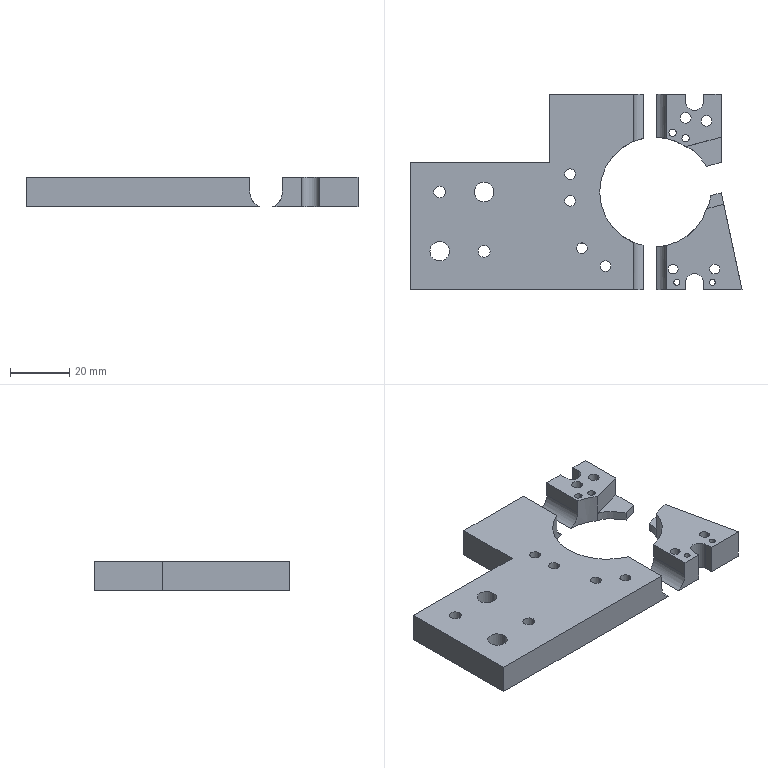Part | SolidWorks | features ICE 6, Extrusion 1 | 3 solids | 75 faces | box 112 x 66 x 10 mm | volume 42287 mm3 | cylinder 42 | plane 31 | spline 2 | commonest cylinder face diameters 3.6 x12 2 x4 2.5 x4 3.3 x4 4 x4 6.6 x4